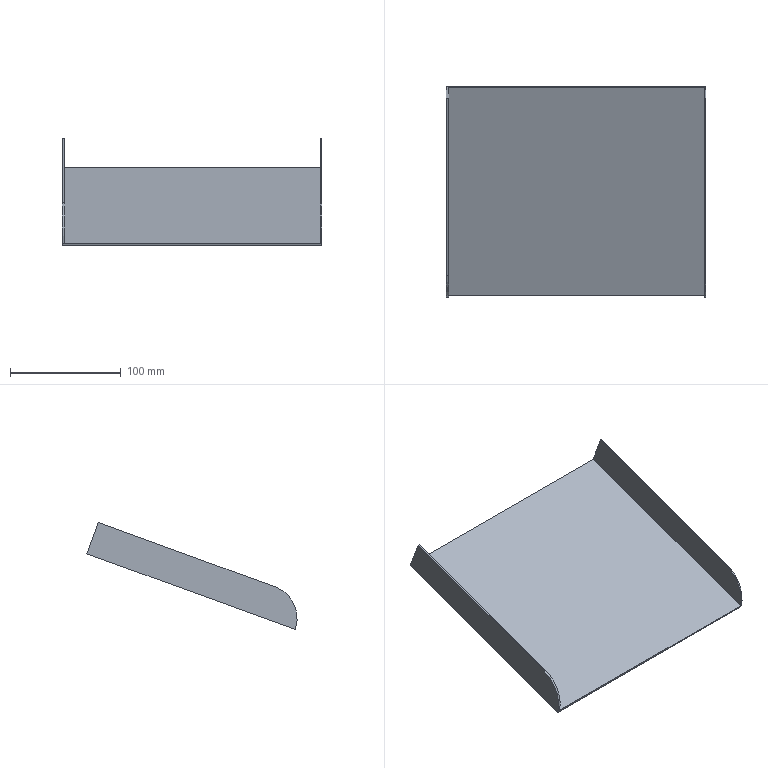Part | NX | features solid 2 | 1 solid | 12 faces | box 234.206 x 189.748 x 96.595 mm | volume 109903 mm3 | plane 10 | cylinder 2 | commonest cylinder face diameters 60 x2
STEP:
#1=CARTESIAN_POINT('',(-1041.794,-810.,-504.758));
#2=VERTEX_POINT('',#1);
#3=CARTESIAN_POINT('',(-1041.794,-997.876,-573.139));
#4=VERTEX_POINT('',#3);
#5=CARTESIAN_POINT('',(-1041.794,-838.191,-515.018));
#6=DIRECTION('',(0.,-0.9397,-0.342));
#7=VECTOR('',#6,1000.);
#8=LINE('',#5,#7);
#9=EDGE_CURVE('',#2,#4,#8,.T.);
#10=ORIENTED_EDGE('',*,*,#9,.F.);
#11=CARTESIAN_POINT('',(-1273.,-810.,-504.758));
#12=VERTEX_POINT('',#11);
#13=CARTESIAN_POINT('',(-1052.794,-810.,-504.758));
#14=DIRECTION('',(-1.,0.,0.));
#15=VECTOR('',#14,1000.);
#16=LINE('',#13,#15);
#17=EDGE_CURVE('',#2,#12,#16,.T.);
#18=ORIENTED_EDGE('',*,*,#17,.T.);
#19=CARTESIAN_POINT('',(-1273.,-997.876,-573.139));
#20=VERTEX_POINT('',#19);
#21=CARTESIAN_POINT('',(-1273.,-838.191,-515.018));
#22=DIRECTION('',(0.,-0.9397,-0.342));
#23=VECTOR('',#22,1000.);
#24=LINE('',#21,#23);
#25=EDGE_CURVE('',#12,#20,#24,.T.);
#26=ORIENTED_EDGE('',*,*,#25,.T.);
#27=CARTESIAN_POINT('',(-1275.,-997.876,-573.139));
#28=VERTEX_POINT('',#27);
#29=CARTESIAN_POINT('',(-1275.,-997.876,-573.139));
#30=DIRECTION('',(-1.,0.,0.));
#31=VECTOR('',#30,1000.);
#32=LINE('',#29,#31);
#33=EDGE_CURVE('',#28,#20,#32,.F.);
#34=ORIENTED_EDGE('',*,*,#33,.F.);
#35=CARTESIAN_POINT('',(-1275.,-997.939,-573.162));
#36=VERTEX_POINT('',#35);
#37=CARTESIAN_POINT('',(-1275.,-838.191,-515.018));
#38=DIRECTION('',(0.,-0.9397,-0.342));
#39=VECTOR('',#38,1000.);
#40=LINE('',#37,#39);
#41=EDGE_CURVE('',#28,#36,#40,.T.);
#42=ORIENTED_EDGE('',*,*,#41,.T.);
#43=CARTESIAN_POINT('',(-1040.794,-997.939,-573.162));
#44=VERTEX_POINT('',#43);
#45=CARTESIAN_POINT('',(-1052.794,-997.939,-573.162));
#46=DIRECTION('',(-1.,0.,0.));
#47=VECTOR('',#46,1000.);
#48=LINE('',#45,#47);
#49=EDGE_CURVE('',#44,#36,#48,.T.);
#50=ORIENTED_EDGE('',*,*,#49,.F.);
#51=CARTESIAN_POINT('',(-1040.794,-997.876,-573.139));
#52=VERTEX_POINT('',#51);
#53=CARTESIAN_POINT('',(-1040.794,-838.191,-515.018));
#54=DIRECTION('',(0.,0.9397,0.342));
#55=VECTOR('',#54,1000.);
#56=LINE('',#53,#55);
#57=EDGE_CURVE('',#52,#44,#56,.F.);
#58=ORIENTED_EDGE('',*,*,#57,.F.);
#59=CARTESIAN_POINT('',(-1040.794,-997.876,-573.139));
#60=DIRECTION('',(1.,0.,0.));
#61=VECTOR('',#60,1000.);
#62=LINE('',#59,#61);
#63=EDGE_CURVE('',#4,#52,#62,.T.);
#64=ORIENTED_EDGE('',*,*,#63,.F.);
#65=EDGE_LOOP('',(#10,#18,#26,#34,#42,#50,#58,#64));
#66=FACE_BOUND('',#65,.T.);
#67=CARTESIAN_POINT('',(-1052.794,-838.191,-515.018));
#68=DIRECTION('',(0.,-0.342,0.9397));
#69=DIRECTION('',(1.,0.,0.));
#70=AXIS2_PLACEMENT_3D('',#67,#68,#69);
#71=PLANE('',#70);
#72=ADVANCED_FACE('',(#66),#71,.T.);
#73=ORIENTED_EDGE('',*,*,#17,.F.);
#74=CARTESIAN_POINT('',(-1041.794,-819.577,-478.446));
#75=VERTEX_POINT('',#74);
#76=CARTESIAN_POINT('',(-1041.794,-809.316,-506.637));
#77=DIRECTION('',(0.,-0.342,0.9397));
#78=VECTOR('',#77,1000.);
#79=LINE('',#76,#78);
#80=EDGE_CURVE('',#2,#75,#79,.T.);
#81=ORIENTED_EDGE('',*,*,#80,.T.);
#82=CARTESIAN_POINT('',(-1040.794,-819.577,-478.446));
#83=VERTEX_POINT('',#82);
#84=CARTESIAN_POINT('',(-1040.794,-819.577,-478.446));
#85=DIRECTION('',(-1.,0.,0.));
#86=VECTOR('',#85,1000.);
#87=LINE('',#84,#86);
#88=EDGE_CURVE('',#83,#75,#87,.T.);
#89=ORIENTED_EDGE('',*,*,#88,.F.);
#90=CARTESIAN_POINT('',(-1040.794,-809.316,-506.637));
#91=VERTEX_POINT('',#90);
#92=CARTESIAN_POINT('',(-1040.794,-810.,-504.758));
#93=DIRECTION('',(0.,-0.342,0.9397));
#94=VECTOR('',#93,1000.);
#95=LINE('',#92,#94);
#96=EDGE_CURVE('',#83,#91,#95,.F.);
#97=ORIENTED_EDGE('',*,*,#96,.T.);
#98=CARTESIAN_POINT('',(-1275.,-809.316,-506.637));
#99=VERTEX_POINT('',#98);
#100=CARTESIAN_POINT('',(-1052.794,-809.316,-506.637));
#101=DIRECTION('',(-1.,0.,0.));
#102=VECTOR('',#101,1000.);
#103=LINE('',#100,#102);
#104=EDGE_CURVE('',#91,#99,#103,.T.);
#105=ORIENTED_EDGE('',*,*,#104,.T.);
#106=CARTESIAN_POINT('',(-1275.,-819.577,-478.446));
#107=VERTEX_POINT('',#106);
#108=CARTESIAN_POINT('',(-1275.,-810.,-504.758));
#109=DIRECTION('',(0.,0.342,-0.9397));
#110=VECTOR('',#109,1000.);
#111=LINE('',#108,#110);
#112=EDGE_CURVE('',#107,#99,#111,.T.);
#113=ORIENTED_EDGE('',*,*,#112,.F.);
#114=CARTESIAN_POINT('',(-1273.,-819.577,-478.446));
#115=VERTEX_POINT('',#114);
#116=CARTESIAN_POINT('',(-1275.,-819.577,-478.446));
#117=DIRECTION('',(-1.,0.,0.));
#118=VECTOR('',#117,1000.);
#119=LINE('',#116,#118);
#120=EDGE_CURVE('',#107,#115,#119,.F.);
#121=ORIENTED_EDGE('',*,*,#120,.T.);
#122=CARTESIAN_POINT('',(-1273.,-809.316,-506.637));
#123=DIRECTION('',(0.,-0.342,0.9397));
#124=VECTOR('',#123,1000.);
#125=LINE('',#122,#124);
#126=EDGE_CURVE('',#12,#115,#125,.T.);
#127=ORIENTED_EDGE('',*,*,#126,.F.);
#128=EDGE_LOOP('',(#73,#81,#89,#97,#105,#113,#121,#127));
#129=FACE_BOUND('',#128,.T.);
#130=CARTESIAN_POINT('',(-1052.794,-810.,-504.758));
#131=DIRECTION('',(0.,0.9397,0.342));
#132=DIRECTION('',(-1.,0.,0.));
#133=AXIS2_PLACEMENT_3D('',#130,#131,#132);
#134=PLANE('',#133);
#135=ADVANCED_FACE('',(#129),#134,.T.);
#136=CARTESIAN_POINT('',(-1040.794,-997.254,-575.041));
#137=VERTEX_POINT('',#136);
#138=CARTESIAN_POINT('',(-1040.794,-997.939,-573.162));
#139=DIRECTION('',(0.,0.342,-0.9397));
#140=VECTOR('',#139,1000.);
#141=LINE('',#138,#140);
#142=EDGE_CURVE('',#44,#137,#141,.T.);
#143=ORIENTED_EDGE('',*,*,#142,.T.);
#144=CARTESIAN_POINT('',(-1040.794,-837.507,-516.898));
#145=DIRECTION('',(0.,0.9397,0.342));
#146=VECTOR('',#145,1000.);
#147=LINE('',#144,#146);
#148=EDGE_CURVE('',#91,#137,#147,.F.);
#149=ORIENTED_EDGE('',*,*,#148,.F.);
#150=ORIENTED_EDGE('',*,*,#96,.F.);
#151=CARTESIAN_POINT('',(-1040.794,-979.324,-536.59));
#152=VERTEX_POINT('',#151);
#153=CARTESIAN_POINT('',(-1040.794,-819.577,-478.446));
#154=DIRECTION('',(0.,-0.9397,-0.342));
#155=VECTOR('',#154,1000.);
#156=LINE('',#153,#155);
#157=EDGE_CURVE('',#83,#152,#156,.T.);
#158=ORIENTED_EDGE('',*,*,#157,.T.);
#159=CARTESIAN_POINT('',(-1040.794,-969.064,-564.78));
#160=DIRECTION('',(-1.,0.,0.));
#161=DIRECTION('',(0.,-0.342,0.9397));
#162=AXIS2_PLACEMENT_3D('',#159,#160,#161);
#163=CIRCLE('',#162,30.);
#164=EDGE_CURVE('',#152,#52,#163,.F.);
#165=ORIENTED_EDGE('',*,*,#164,.T.);
#166=ORIENTED_EDGE('',*,*,#57,.T.);
#167=EDGE_LOOP('',(#143,#149,#150,#158,#165,#166));
#168=FACE_BOUND('',#167,.T.);
#169=CARTESIAN_POINT('',(-1040.794,-838.191,-515.018));
#170=DIRECTION('',(-1.,0.,0.));
#171=DIRECTION('',(0.,-0.9397,-0.342));
#172=AXIS2_PLACEMENT_3D('',#169,#170,#171);
#173=PLANE('',#172);
#174=ADVANCED_FACE('',(#168),#173,.F.);
#175=ORIENTED_EDGE('',*,*,#142,.F.);
#176=ORIENTED_EDGE('',*,*,#49,.T.);
#177=CARTESIAN_POINT('',(-1275.,-997.254,-575.041));
#178=VERTEX_POINT('',#177);
#179=CARTESIAN_POINT('',(-1275.,-997.939,-573.162));
#180=DIRECTION('',(0.,-0.342,0.9397));
#181=VECTOR('',#180,1000.);
#182=LINE('',#179,#181);
#183=EDGE_CURVE('',#36,#178,#182,.F.);
#184=ORIENTED_EDGE('',*,*,#183,.T.);
#185=CARTESIAN_POINT('',(-1052.794,-997.254,-575.041));
#186=DIRECTION('',(1.,0.,0.));
#187=VECTOR('',#186,1000.);
#188=LINE('',#185,#187);
#189=EDGE_CURVE('',#137,#178,#188,.F.);
#190=ORIENTED_EDGE('',*,*,#189,.F.);
#191=EDGE_LOOP('',(#175,#176,#184,#190));
#192=FACE_BOUND('',#191,.T.);
#193=CARTESIAN_POINT('',(-1052.794,-997.939,-573.162));
#194=DIRECTION('',(0.,0.9397,0.342));
#195=DIRECTION('',(-1.,0.,0.));
#196=AXIS2_PLACEMENT_3D('',#193,#194,#195);
#197=PLANE('',#196);
#198=ADVANCED_FACE('',(#192),#197,.F.);
#199=CARTESIAN_POINT('',(-1275.,-837.507,-516.898));
#200=DIRECTION('',(0.,-0.9397,-0.342));
#201=VECTOR('',#200,1000.);
#202=LINE('',#199,#201);
#203=EDGE_CURVE('',#99,#178,#202,.T.);
#204=ORIENTED_EDGE('',*,*,#203,.F.);
#205=ORIENTED_EDGE('',*,*,#104,.F.);
#206=ORIENTED_EDGE('',*,*,#148,.T.);
#207=ORIENTED_EDGE('',*,*,#189,.T.);
#208=EDGE_LOOP('',(#204,#205,#206,#207));
#209=FACE_BOUND('',#208,.T.);
#210=CARTESIAN_POINT('',(-1052.794,-837.507,-516.898));
#211=DIRECTION('',(0.,-0.342,0.9397));
#212=DIRECTION('',(1.,0.,0.));
#213=AXIS2_PLACEMENT_3D('',#210,#211,#212);
#214=PLANE('',#213);
#215=ADVANCED_FACE('',(#209),#214,.F.);
#216=ORIENTED_EDGE('',*,*,#41,.F.);
#217=CARTESIAN_POINT('',(-1275.,-979.324,-536.59));
#218=VERTEX_POINT('',#217);
#219=CARTESIAN_POINT('',(-1275.,-969.064,-564.78));
#220=DIRECTION('',(-1.,0.,0.));
#221=DIRECTION('',(0.,-0.342,0.9397));
#222=AXIS2_PLACEMENT_3D('',#219,#220,#221);
#223=CIRCLE('',#222,30.);
#224=EDGE_CURVE('',#28,#218,#223,.T.);
#225=ORIENTED_EDGE('',*,*,#224,.T.);
#226=CARTESIAN_POINT('',(-1275.,-819.577,-478.446));
#227=DIRECTION('',(0.,-0.9397,-0.342));
#228=VECTOR('',#227,1000.);
#229=LINE('',#226,#228);
#230=EDGE_CURVE('',#107,#218,#229,.T.);
#231=ORIENTED_EDGE('',*,*,#230,.F.);
#232=ORIENTED_EDGE('',*,*,#112,.T.);
#233=ORIENTED_EDGE('',*,*,#203,.T.);
#234=ORIENTED_EDGE('',*,*,#183,.F.);
#235=EDGE_LOOP('',(#216,#225,#231,#232,#233,#234));
#236=FACE_BOUND('',#235,.T.);
#237=CARTESIAN_POINT('',(-1275.,-838.191,-515.018));
#238=DIRECTION('',(-1.,0.,0.));
#239=DIRECTION('',(0.,-0.9397,-0.342));
#240=AXIS2_PLACEMENT_3D('',#237,#238,#239);
#241=PLANE('',#240);
#242=ADVANCED_FACE('',(#236),#241,.T.);
#243=ORIENTED_EDGE('',*,*,#230,.T.);
#244=CARTESIAN_POINT('',(-1273.,-979.324,-536.59));
#245=VERTEX_POINT('',#244);
#246=CARTESIAN_POINT('',(-1275.,-979.324,-536.59));
#247=DIRECTION('',(-1.,0.,0.));
#248=VECTOR('',#247,1000.);
#249=LINE('',#246,#248);
#250=EDGE_CURVE('',#218,#245,#249,.F.);
#251=ORIENTED_EDGE('',*,*,#250,.T.);
#252=CARTESIAN_POINT('',(-1273.,-819.577,-478.446));
#253=DIRECTION('',(0.,0.9397,0.342));
#254=VECTOR('',#253,1000.);
#255=LINE('',#252,#254);
#256=EDGE_CURVE('',#115,#245,#255,.F.);
#257=ORIENTED_EDGE('',*,*,#256,.F.);
#258=ORIENTED_EDGE('',*,*,#120,.F.);
#259=EDGE_LOOP('',(#243,#251,#257,#258));
#260=FACE_BOUND('',#259,.T.);
#261=CARTESIAN_POINT('',(-1275.,-819.577,-478.446));
#262=DIRECTION('',(0.,0.342,-0.9397));
#263=DIRECTION('',(0.,-0.9397,-0.342));
#264=AXIS2_PLACEMENT_3D('',#261,#262,#263);
#265=PLANE('',#264);
#266=ADVANCED_FACE('',(#260),#265,.F.);
#267=ORIENTED_EDGE('',*,*,#25,.F.);
#268=ORIENTED_EDGE('',*,*,#126,.T.);
#269=ORIENTED_EDGE('',*,*,#256,.T.);
#270=CARTESIAN_POINT('',(-1273.,-969.064,-564.78));
#271=DIRECTION('',(-1.,0.,0.));
#272=DIRECTION('',(0.,-0.342,0.9397));
#273=AXIS2_PLACEMENT_3D('',#270,#271,#272);
#274=CIRCLE('',#273,30.);
#275=EDGE_CURVE('',#245,#20,#274,.F.);
#276=ORIENTED_EDGE('',*,*,#275,.T.);
#277=EDGE_LOOP('',(#267,#268,#269,#276));
#278=FACE_BOUND('',#277,.T.);
#279=CARTESIAN_POINT('',(-1273.,-809.316,-506.637));
#280=DIRECTION('',(-1.,0.,0.));
#281=DIRECTION('',(0.,-0.342,0.9397));
#282=AXIS2_PLACEMENT_3D('',#279,#280,#281);
#283=PLANE('',#282);
#284=ADVANCED_FACE('',(#278),#283,.F.);
#285=ORIENTED_EDGE('',*,*,#224,.F.);
#286=ORIENTED_EDGE('',*,*,#33,.T.);
#287=ORIENTED_EDGE('',*,*,#275,.F.);
#288=ORIENTED_EDGE('',*,*,#250,.F.);
#289=EDGE_LOOP('',(#285,#286,#287,#288));
#290=FACE_BOUND('',#289,.T.);
#291=CARTESIAN_POINT('',(-1275.,-969.064,-564.78));
#292=DIRECTION('',(-1.,0.,0.));
#293=DIRECTION('',(0.,-0.342,0.9397));
#294=AXIS2_PLACEMENT_3D('',#291,#292,#293);
#295=CYLINDRICAL_SURFACE('',#294,30.);
#296=ADVANCED_FACE('',(#290),#295,.T.);
#297=CARTESIAN_POINT('',(-1041.794,-979.324,-536.59));
#298=VERTEX_POINT('',#297);
#299=CARTESIAN_POINT('',(-1041.794,-819.577,-478.446));
#300=DIRECTION('',(0.,0.9397,0.342));
#301=VECTOR('',#300,1000.);
#302=LINE('',#299,#301);
#303=EDGE_CURVE('',#75,#298,#302,.F.);
#304=ORIENTED_EDGE('',*,*,#303,.T.);
#305=CARTESIAN_POINT('',(-1040.794,-979.324,-536.59));
#306=DIRECTION('',(-1.,0.,0.));
#307=VECTOR('',#306,1000.);
#308=LINE('',#305,#307);
#309=EDGE_CURVE('',#298,#152,#308,.F.);
#310=ORIENTED_EDGE('',*,*,#309,.T.);
#311=ORIENTED_EDGE('',*,*,#157,.F.);
#312=ORIENTED_EDGE('',*,*,#88,.T.);
#313=EDGE_LOOP('',(#304,#310,#311,#312));
#314=FACE_BOUND('',#313,.T.);
#315=CARTESIAN_POINT('',(-1040.794,-819.577,-478.446));
#316=DIRECTION('',(0.,0.342,-0.9397));
#317=DIRECTION('',(0.,-0.9397,-0.342));
#318=AXIS2_PLACEMENT_3D('',#315,#316,#317);
#319=PLANE('',#318);
#320=ADVANCED_FACE('',(#314),#319,.F.);
#321=ORIENTED_EDGE('',*,*,#80,.F.);
#322=ORIENTED_EDGE('',*,*,#9,.T.);
#323=CARTESIAN_POINT('',(-1041.794,-969.064,-564.78));
#324=DIRECTION('',(-1.,0.,0.));
#325=DIRECTION('',(0.,-0.342,0.9397));
#326=AXIS2_PLACEMENT_3D('',#323,#324,#325);
#327=CIRCLE('',#326,30.);
#328=EDGE_CURVE('',#4,#298,#327,.T.);
#329=ORIENTED_EDGE('',*,*,#328,.T.);
#330=ORIENTED_EDGE('',*,*,#303,.F.);
#331=EDGE_LOOP('',(#321,#322,#329,#330));
#332=FACE_BOUND('',#331,.T.);
#333=CARTESIAN_POINT('',(-1041.794,-809.316,-506.637));
#334=DIRECTION('',(-1.,0.,0.));
#335=DIRECTION('',(0.,-0.342,0.9397));
#336=AXIS2_PLACEMENT_3D('',#333,#334,#335);
#337=PLANE('',#336);
#338=ADVANCED_FACE('',(#332),#337,.T.);
#339=ORIENTED_EDGE('',*,*,#328,.F.);
#340=ORIENTED_EDGE('',*,*,#63,.T.);
#341=ORIENTED_EDGE('',*,*,#164,.F.);
#342=ORIENTED_EDGE('',*,*,#309,.F.);
#343=EDGE_LOOP('',(#339,#340,#341,#342));
#344=FACE_BOUND('',#343,.T.);
#345=CARTESIAN_POINT('',(-1040.794,-969.064,-564.78));
#346=DIRECTION('',(1.,0.,0.));
#347=DIRECTION('',(0.,0.342,-0.9397));
#348=AXIS2_PLACEMENT_3D('',#345,#346,#347);
#349=CYLINDRICAL_SURFACE('',#348,30.);
#350=ADVANCED_FACE('',(#344),#349,.T.);
#351=CLOSED_SHELL('',(#72,#135,#174,#198,#215,#242,#266,#284,#296,#320,#338,#350));
#352=MANIFOLD_SOLID_BREP('',#351);
#353=(LENGTH_UNIT()NAMED_UNIT(*)SI_UNIT(.MILLI.,.METRE.));
#354=UNCERTAINTY_MEASURE_WITH_UNIT(LENGTH_MEASURE(0.00001),#353,'','');
#355=(NAMED_UNIT(*)PLANE_ANGLE_UNIT()SI_UNIT($,.RADIAN.));
#356=(NAMED_UNIT(*)SI_UNIT($,.STERADIAN.)SOLID_ANGLE_UNIT());
#357=(GEOMETRIC_REPRESENTATION_CONTEXT(3)GLOBAL_UNCERTAINTY_ASSIGNED_CONTEXT((#354))GLOBAL_UNIT_ASSIGNED_CONTEXT((#353,#355,#356))REPRESENTATION_CONTEXT('',''));
#358=ADVANCED_BREP_SHAPE_REPRESENTATION('',(#352),#357);